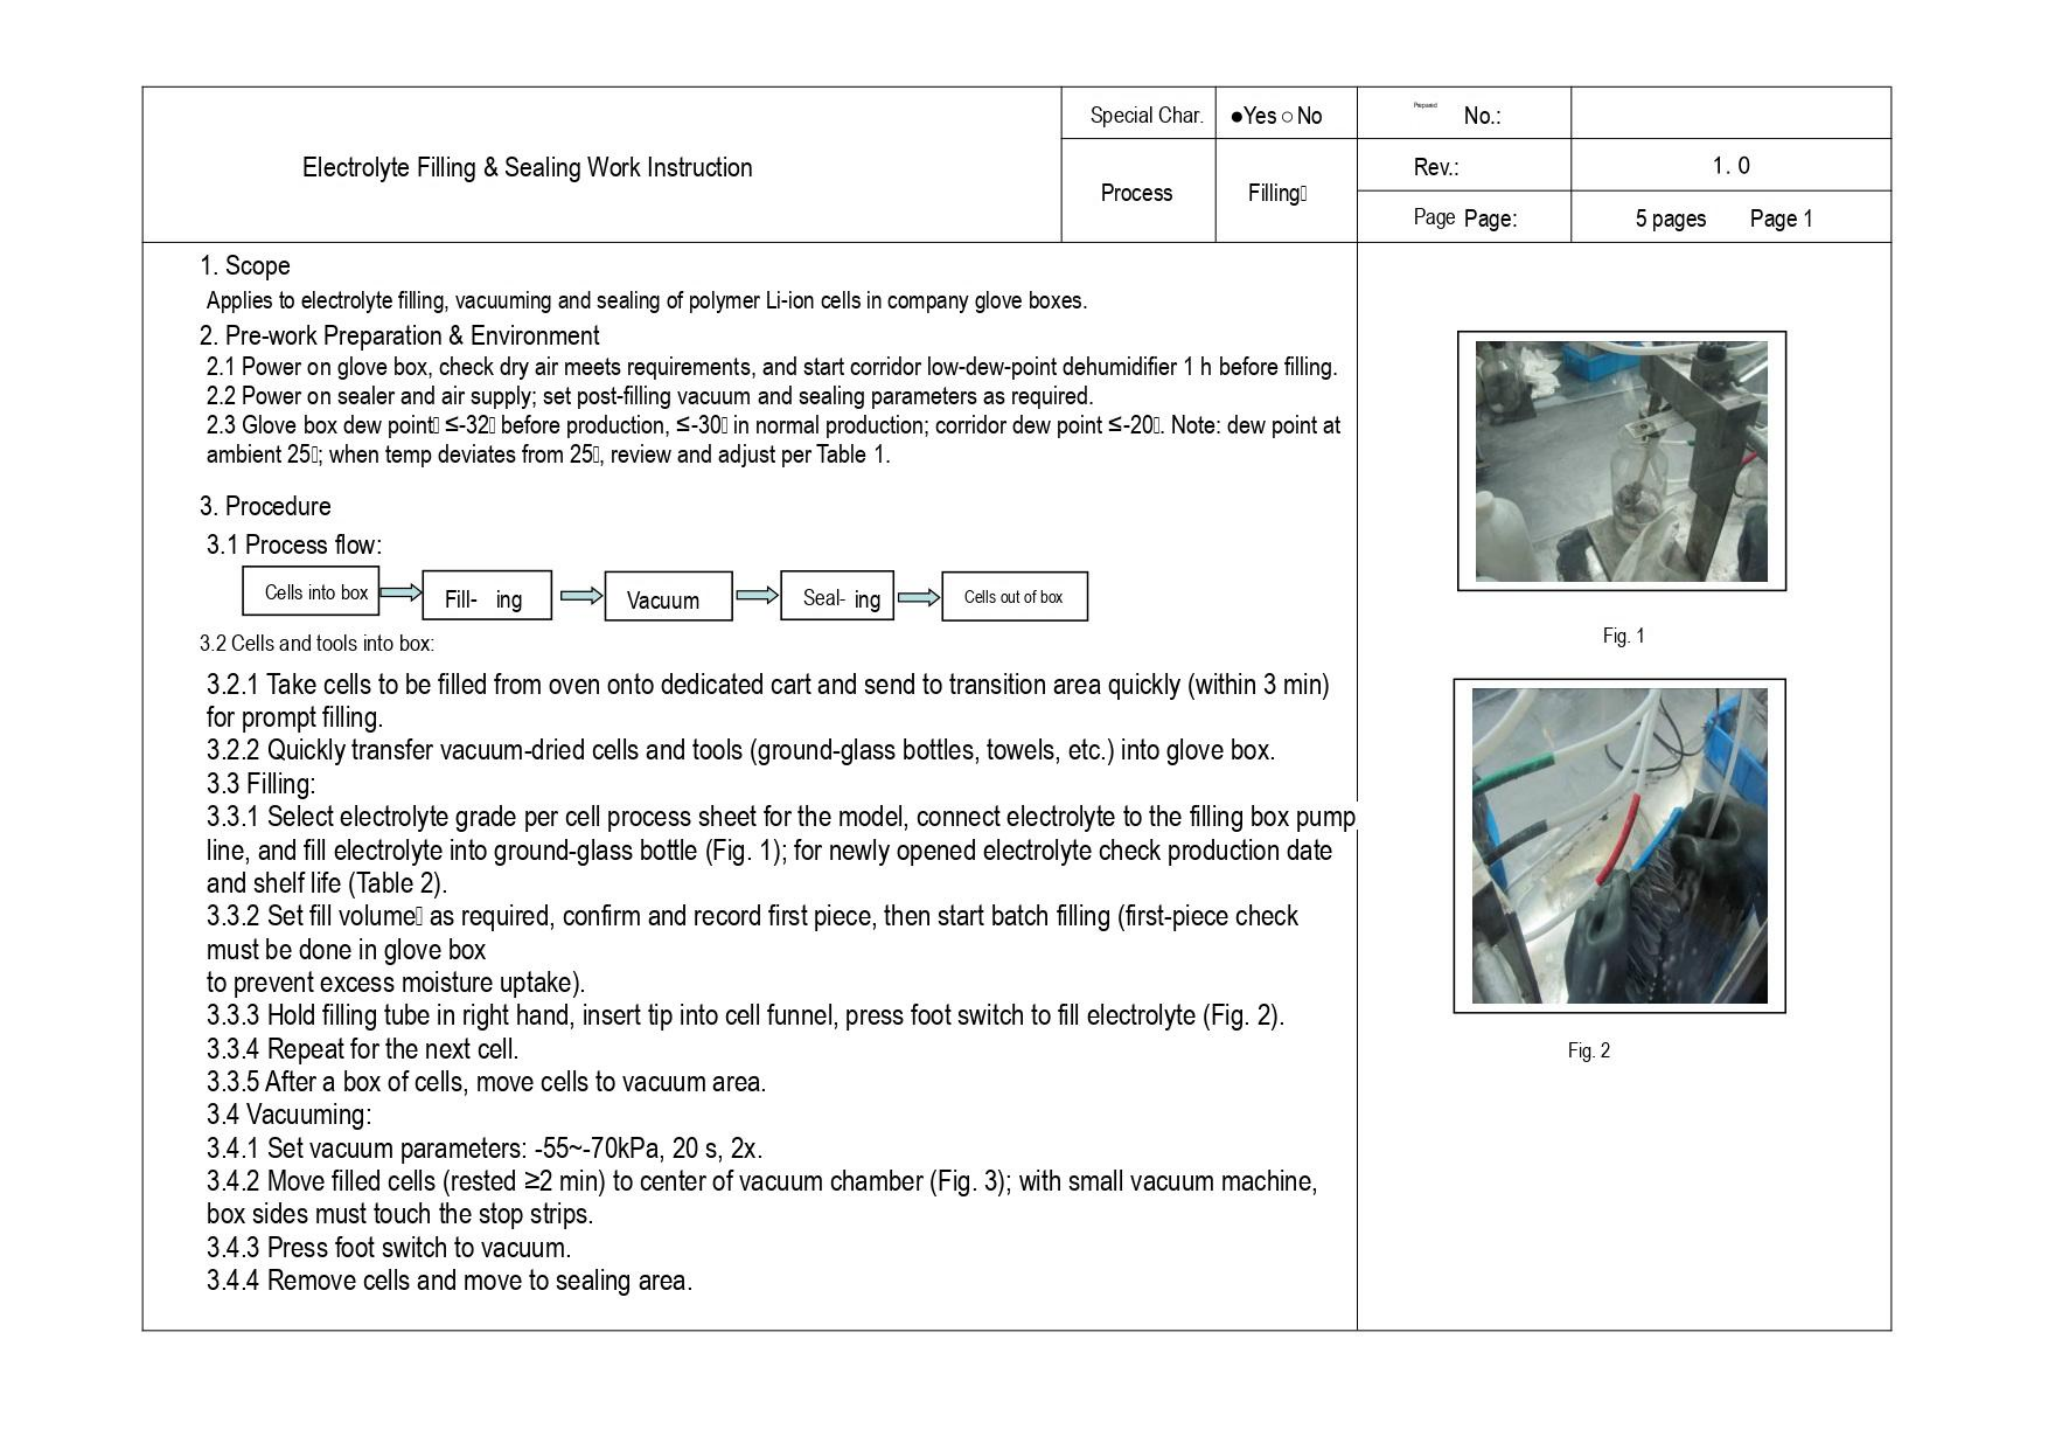| Electrolyte Filling & Sealing Work Instruction | Special Char. | ●Yes ○ No | No.: | |
|---|---|---|---|---|
| | Process | Filling | Rev.: | 1. 0 |
| | | | Page Page: | 5 pages Page 1 |

1. Scope
Applies to electrolyte filling, vacuuming and sealing of polymer Li-ion cells in company glove boxes.

2. Pre-work Preparation & Environment
2.1 Power on glove box, check dry air meets requirements, and start corridor low-dew-point dehumidifier 1 h before filling.
2.2 Power on sealer and air supply; set post-filling vacuum and sealing parameters as required.
2.3 Glove box dew point ≤-32 before production, ≤-30 in normal production; corridor dew point ≤-20. Note: dew point at ambient 25; when temp deviates from 25, review and adjust per Table 1.

3. Procedure
3.1 Process flow:
Cells into box → Fill- ing → Vacuum → Seal- ing → Cells out of box
3.2 Cells and tools into box:
3.2.1 Take cells to be filled from oven onto dedicated cart and send to transition area quickly (within 3 min) for prompt filling.
3.2.2 Quickly transfer vacuum-dried cells and tools (ground-glass bottles, towels, etc.) into glove box.
3.3 Filling:
3.3.1 Select electrolyte grade per cell process sheet for the model, connect electrolyte to the filling box pump line, and fill electrolyte into ground-glass bottle (Fig. 1); for newly opened electrolyte check production date and shelf life (Table 2).
3.3.2 Set fill volume as required, confirm and record first piece, then start batch filling (first-piece check must be done in glove box
to prevent excess moisture uptake).
3.3.3 Hold filling tube in right hand, insert tip into cell funnel, press foot switch to fill electrolyte (Fig. 2).
3.3.4 Repeat for the next cell.
3.3.5 After a box of cells, move cells to vacuum area.
3.4 Vacuuming:
3.4.1 Set vacuum parameters: -55~-70kPa, 20 s, 2x.
3.4.2 Move filled cells (rested ≥2 min) to center of vacuum chamber (Fig. 3); with small vacuum machine, box sides must touch the stop strips.
3.4.3 Press foot switch to vacuum.
3.4.4 Remove cells and move to sealing area.

Fig. 1

Fig. 2
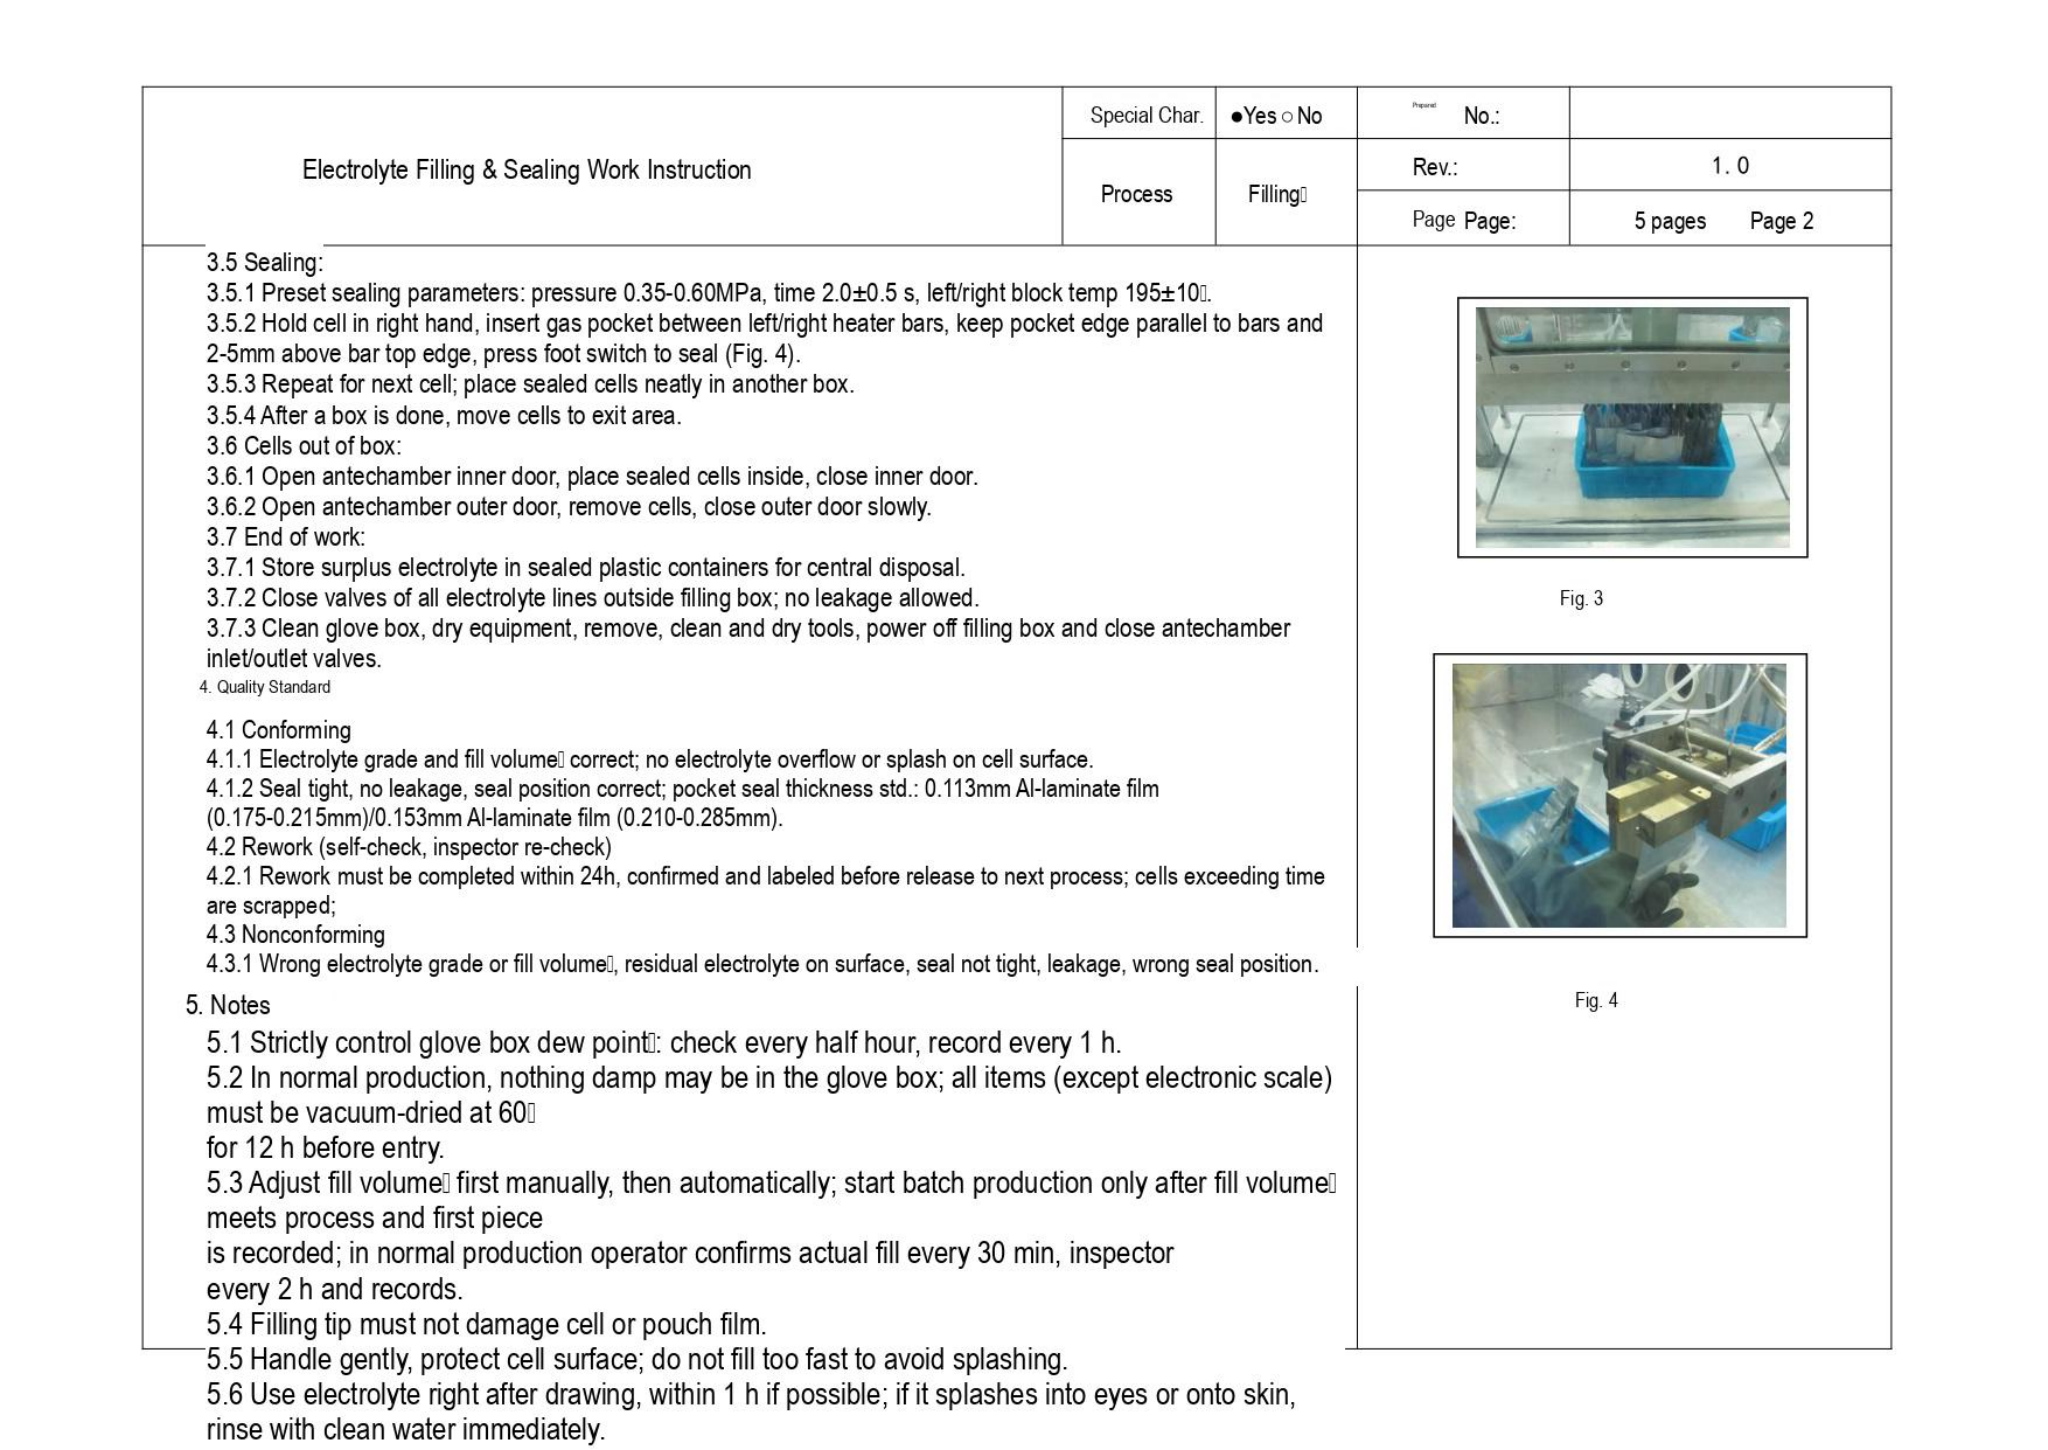| Electrolyte Filling & Sealing Work Instruction | Special Char. | ●Yes ○ No | No.: | |
|---|---|---|---|---|
| | Process | Filling | Rev.: | 1. 0 |
| | | | Page Page: | 5 pages Page 2 |

3.5 Sealing:
3.5.1 Preset sealing parameters: pressure 0.35-0.60MPa, time 2.0±0.5 s, left/right block temp 195±10.
3.5.2 Hold cell in right hand, insert gas pocket between left/right heater bars, keep pocket edge parallel to bars and 2-5mm above bar top edge, press foot switch to seal (Fig. 4).
3.5.3 Repeat for next cell; place sealed cells neatly in another box.
3.5.4 After a box is done, move cells to exit area.
3.6 Cells out of box:
3.6.1 Open antechamber inner door, place sealed cells inside, close inner door.
3.6.2 Open antechamber outer door, remove cells, close outer door slowly.
3.7 End of work:
3.7.1 Store surplus electrolyte in sealed plastic containers for central disposal.
3.7.2 Close valves of all electrolyte lines outside filling box; no leakage allowed.
3.7.3 Clean glove box, dry equipment, remove, clean and dry tools, power off filling box and close antechamber inlet/outlet valves.
4. Quality Standard

4.1 Conforming
4.1.1 Electrolyte grade and fill volume correct; no electrolyte overflow or splash on cell surface.
4.1.2 Seal tight, no leakage, seal position correct; pocket seal thickness std.: 0.113mm Al-laminate film (0.175-0.215mm)/0.153mm Al-laminate film (0.210-0.285mm).
4.2 Rework (self-check, inspector re-check)
4.2.1 Rework must be completed within 24h, confirmed and labeled before release to next process; cells exceeding time are scrapped;
4.3 Nonconforming
4.3.1 Wrong electrolyte grade or fill volume, residual electrolyte on surface, seal not tight, leakage, wrong seal position.

Fig. 3

Fig. 4

5. Notes
5.1 Strictly control glove box dew point: check every half hour, record every 1 h.
5.2 In normal production, nothing damp may be in the glove box; all items (except electronic scale) must be vacuum-dried at 60
for 12 h before entry.
5.3 Adjust fill volume first manually, then automatically; start batch production only after fill volume meets process and first piece
is recorded; in normal production operator confirms actual fill every 30 min, inspector
every 2 h and records.
5.4 Filling tip must not damage cell or pouch film.
5.5 Handle gently, protect cell surface; do not fill too fast to avoid splashing.
5.6 Use electrolyte right after drawing, within 1 h if possible; if it splashes into eyes or onto skin, rinse with clean water immediately.
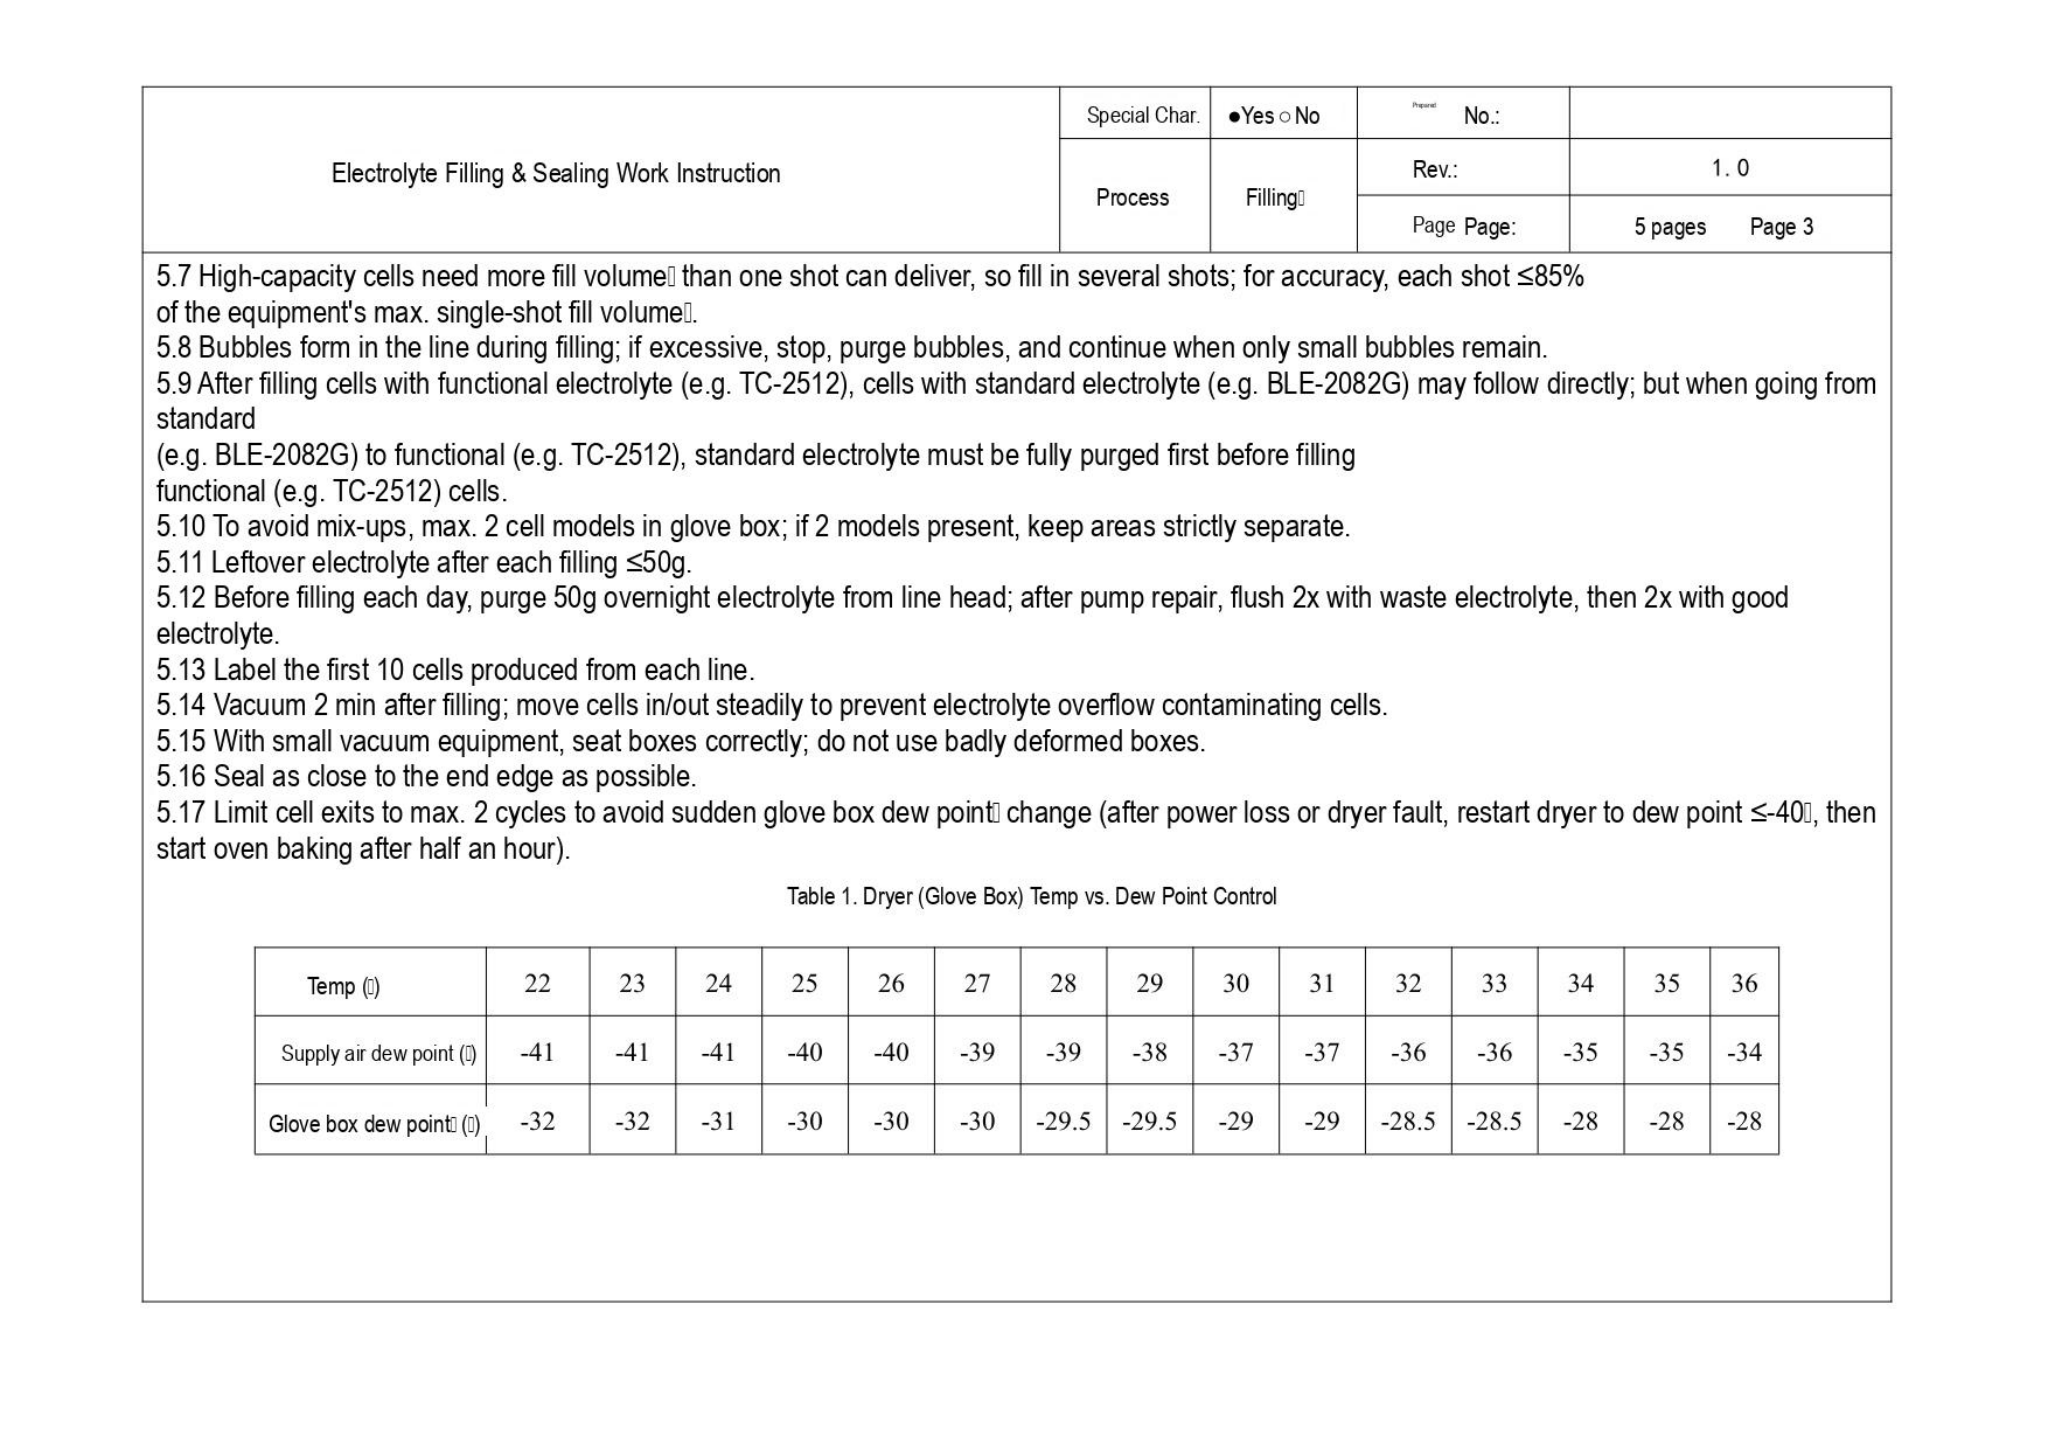| Electrolyte Filling & Sealing Work Instruction | Special Char. | ●Yes ○No | No.: | |
|---|---|---|---|---|
| | Process | Filling | Rev.: | 1. 0 |
| | | | Page Page: | 5 pages Page 3 |

5.7 High-capacity cells need more fill volume than one shot can deliver, so fill in several shots; for accuracy, each shot ≤85% of the equipment's max. single-shot fill volume.
5.8 Bubbles form in the line during filling; if excessive, stop, purge bubbles, and continue when only small bubbles remain.
5.9 After filling cells with functional electrolyte (e.g. TC-2512), cells with standard electrolyte (e.g. BLE-2082G) may follow directly; but when going from standard
(e.g. BLE-2082G) to functional (e.g. TC-2512), standard electrolyte must be fully purged first before filling
functional (e.g. TC-2512) cells.
5.10 To avoid mix-ups, max. 2 cell models in glove box; if 2 models present, keep areas strictly separate.
5.11 Leftover electrolyte after each filling ≤50g.
5.12 Before filling each day, purge 50g overnight electrolyte from line head; after pump repair, flush 2x with waste electrolyte, then 2x with good electrolyte.
5.13 Label the first 10 cells produced from each line.
5.14 Vacuum 2 min after filling; move cells in/out steadily to prevent electrolyte overflow contaminating cells.
5.15 With small vacuum equipment, seat boxes correctly; do not use badly deformed boxes.
5.16 Seal as close to the end edge as possible.
5.17 Limit cell exits to max. 2 cycles to avoid sudden glove box dew point change (after power loss or dryer fault, restart dryer to dew point ≤-40, then start oven baking after half an hour).

Table 1. Dryer (Glove Box) Temp vs. Dew Point Control

| Temp () | 22 | 23 | 24 | 25 | 26 | 27 | 28 | 29 | 30 | 31 | 32 | 33 | 34 | 35 | 36 |
|---|---|---|---|---|---|---|---|---|---|---|---|---|---|---|---|
| Supply air dew point () | -41 | -41 | -41 | -40 | -40 | -39 | -39 | -38 | -37 | -37 | -36 | -36 | -35 | -35 | -34 |
| Glove box dew point () | -32 | -32 | -31 | -30 | -30 | -30 | -29.5 | -29.5 | -29 | -29 | -28.5 | -28.5 | -28 | -28 | -28 |
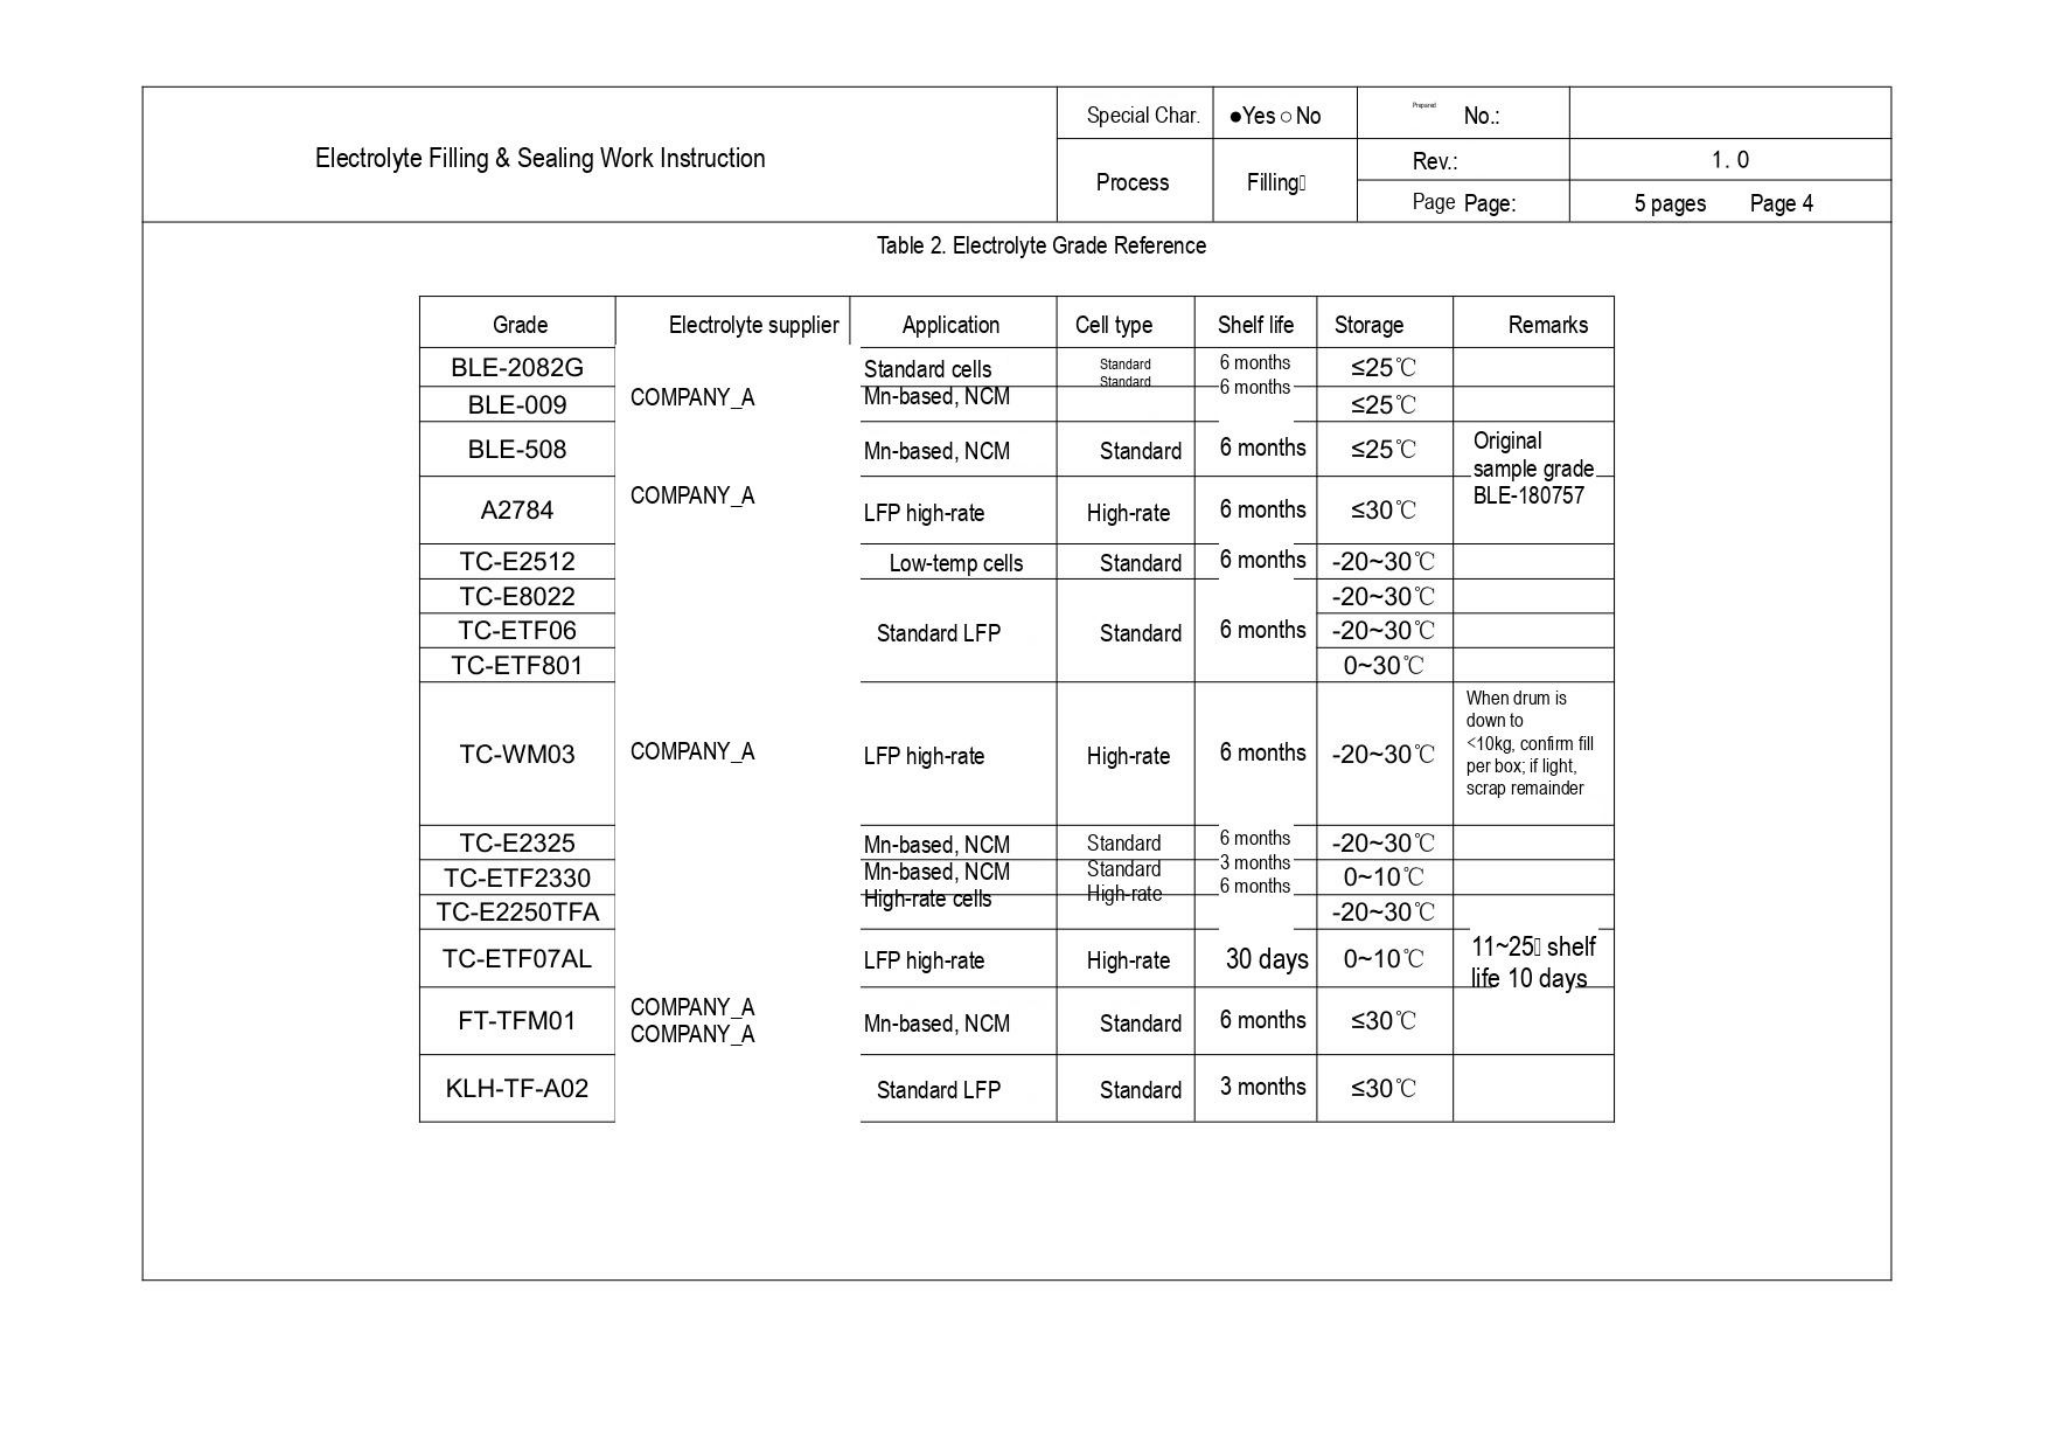# Electrolyte Filling & Sealing Work Instruction

| Electrolyte Filling & Sealing Work Instruction | Special Char. | ●Yes ○No | No.: | |
|---|---|---|---|---|
| | Process | Filling | Rev.: | 1. 0 |
| | | | Page Page: | 5 pages Page 4 |

Table 2. Electrolyte Grade Reference

| Grade | Electrolyte supplier | Application | Cell type | Shelf life | Storage | Remarks |
|---|---|---|---|---|---|---|
| BLE-2082G | COMPANY_A | Standard cells | Standard | 6 months | ≤25℃ | |
| BLE-009 | | Mn-based, NCM | Standard | 6 months | ≤25℃ | |
| BLE-508 | COMPANY_A | Mn-based, NCM | Standard | 6 months | ≤25℃ | Original sample grade BLE-180757 |
| A2784 | | LFP high-rate | High-rate | 6 months | ≤30℃ | |
| TC-E2512 | | Low-temp cells | Standard | 6 months | -20~30℃ | |
| TC-E8022 | | Standard LFP | Standard | 6 months | -20~30℃ | |
| TC-ETF06 | | | | | -20~30℃ | |
| TC-ETF801 | | | | | 0~30℃ | |
| TC-WM03 | COMPANY_A | LFP high-rate | High-rate | 6 months | -20~30℃ | When drum is down to <10kg, confirm fill per box; if light, scrap remainder |
| TC-E2325 | | Mn-based, NCM | Standard | 6 months | -20~30℃ | |
| TC-ETF2330 | | Mn-based, NCM | Standard | 3 months | 0~10℃ | |
| TC-E2250TFA | | High-rate cells | High-rate | 6 months | -20~30℃ | |
| TC-ETF07AL | | LFP high-rate | High-rate | 30 days | 0~10℃ | 11~25 shelf life 10 days |
| FT-TFM01 | COMPANY_A COMPANY_A | Mn-based, NCM | Standard | 6 months | ≤30℃ | |
| KLH-TF-A02 | | Standard LFP | Standard | 3 months | ≤30℃ | |
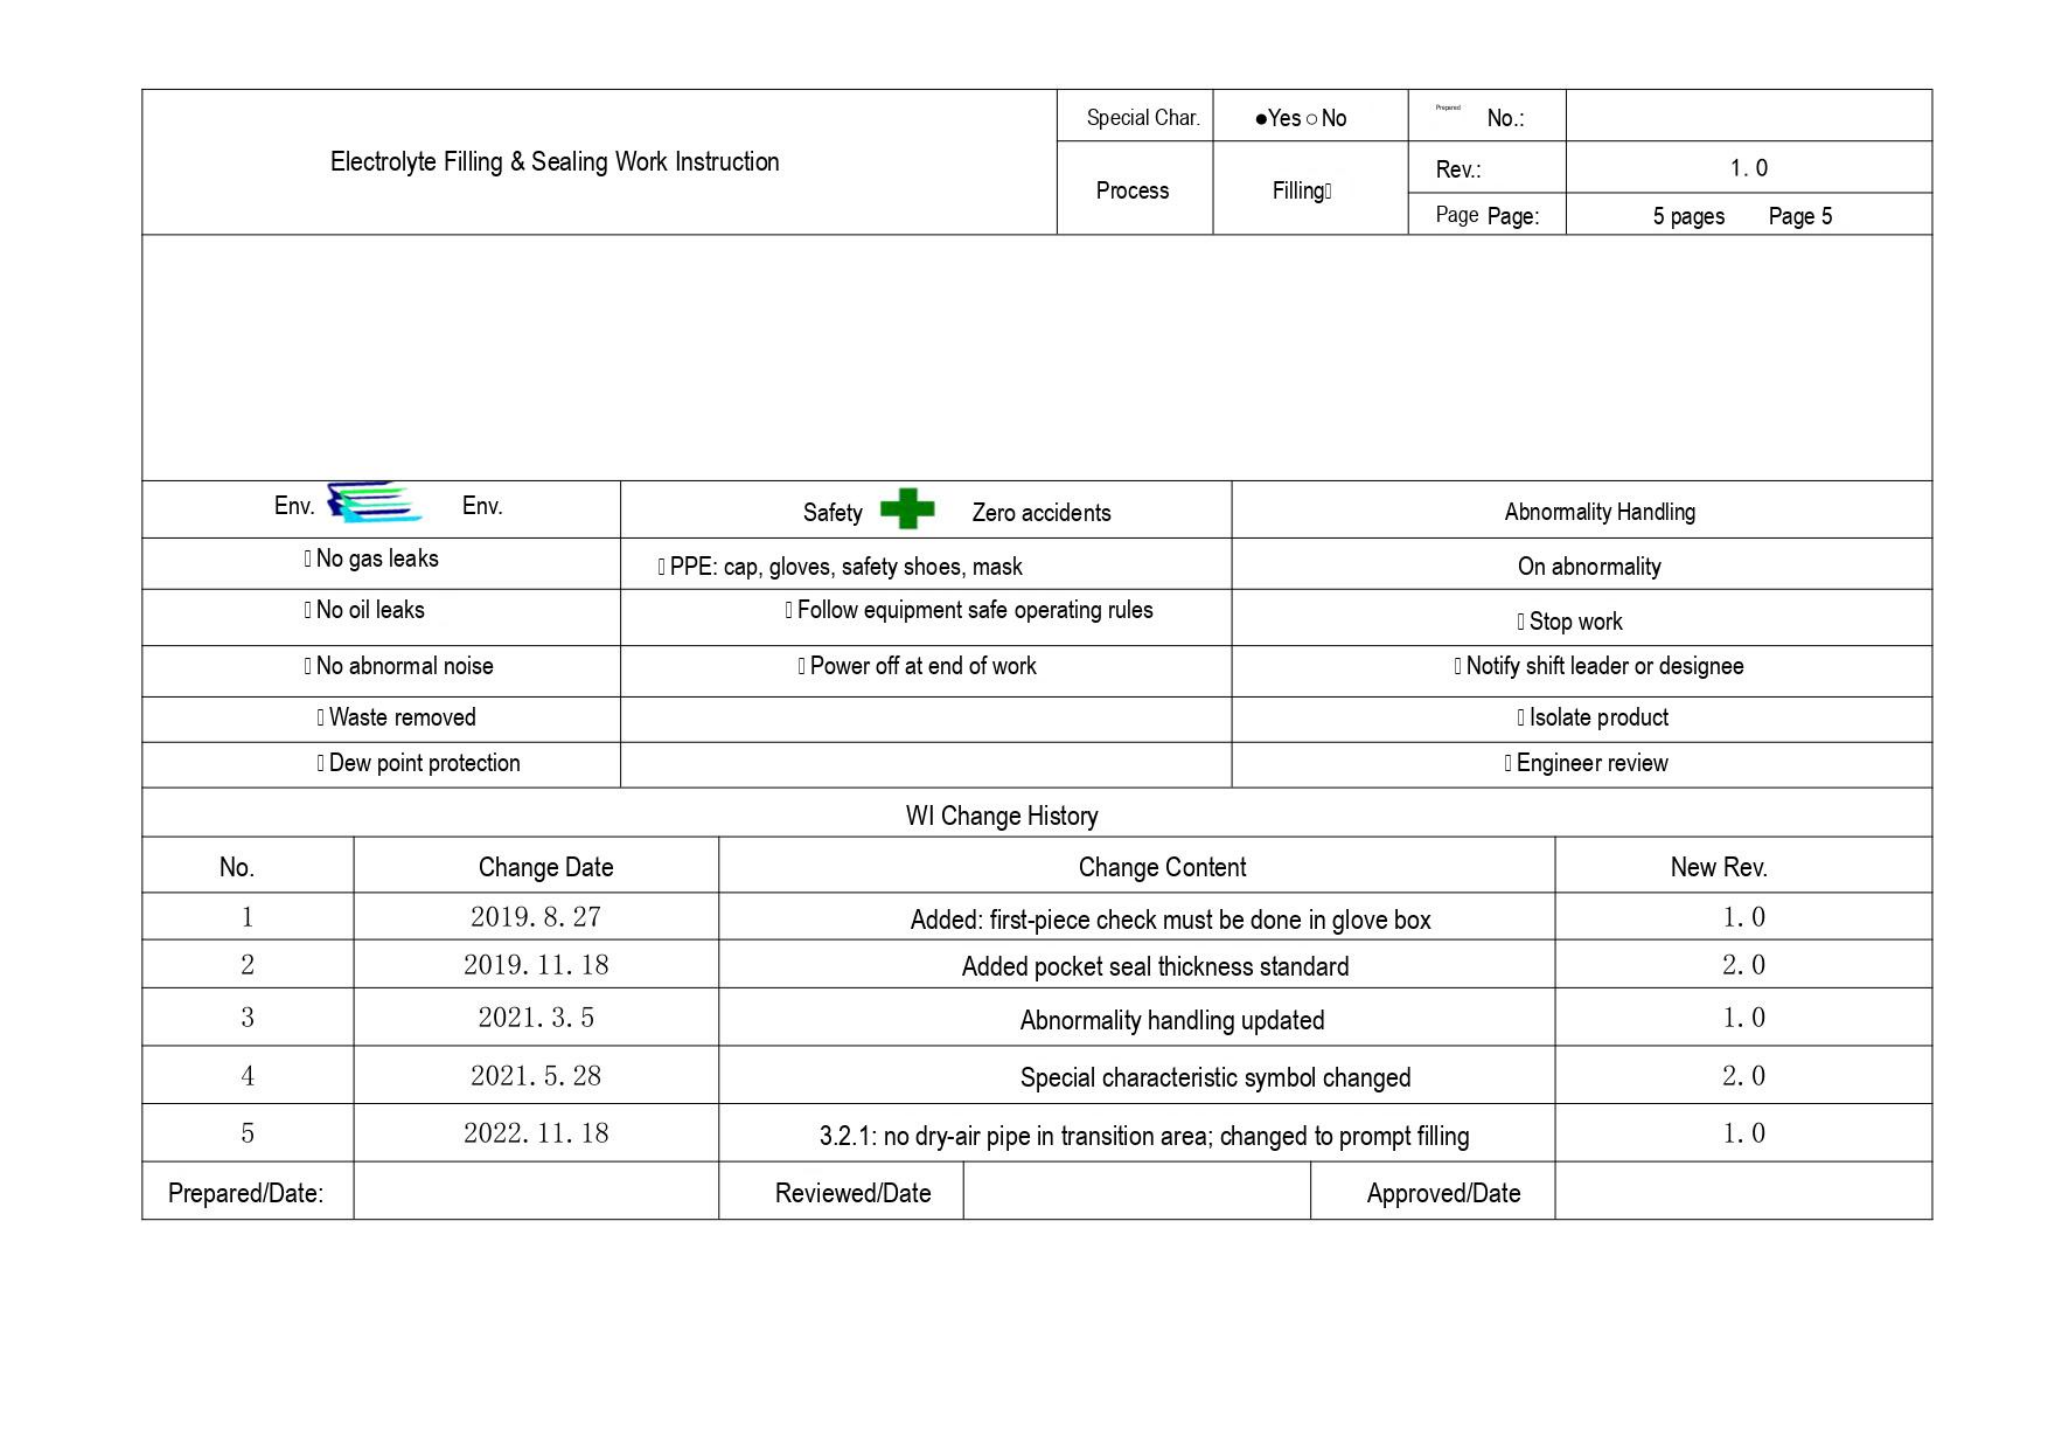| Electrolyte Filling & Sealing Work Instruction | Special Char. | ●Yes ○ No | Prepared No.: | |
|---|---|---|---|---|
| | Process | Filling | Rev.: | 1. 0 |
| | | | Page Page: | 5 pages Page 5 |

| Env. Env. | Safety Zero accidents | Abnormality Handling |
|---|---|---|
| No gas leaks | PPE: cap, gloves, safety shoes, mask | On abnormality |
| No oil leaks | Follow equipment safe operating rules | Stop work |
| No abnormal noise | Power off at end of work | Notify shift leader or designee |
| Waste removed | | Isolate product |
| Dew point protection | | Engineer review |

WI Change History

| No. | Change Date | Change Content | | New Rev. |
|---|---|---|---|---|
| 1 | 2019. 8. 27 | Added: first-piece check must be done in glove box | | 1. 0 |
| 2 | 2019. 11. 18 | Added pocket seal thickness standard | | 2. 0 |
| 3 | 2021. 3. 5 | Abnormality handling updated | | 1. 0 |
| 4 | 2021. 5. 28 | Special characteristic symbol changed | | 2. 0 |
| 5 | 2022. 11. 18 | 3.2.1: no dry-air pipe in transition area; changed to prompt filling | | 1. 0 |
| Prepared/Date: | | Reviewed/Date | Approved/Date | |